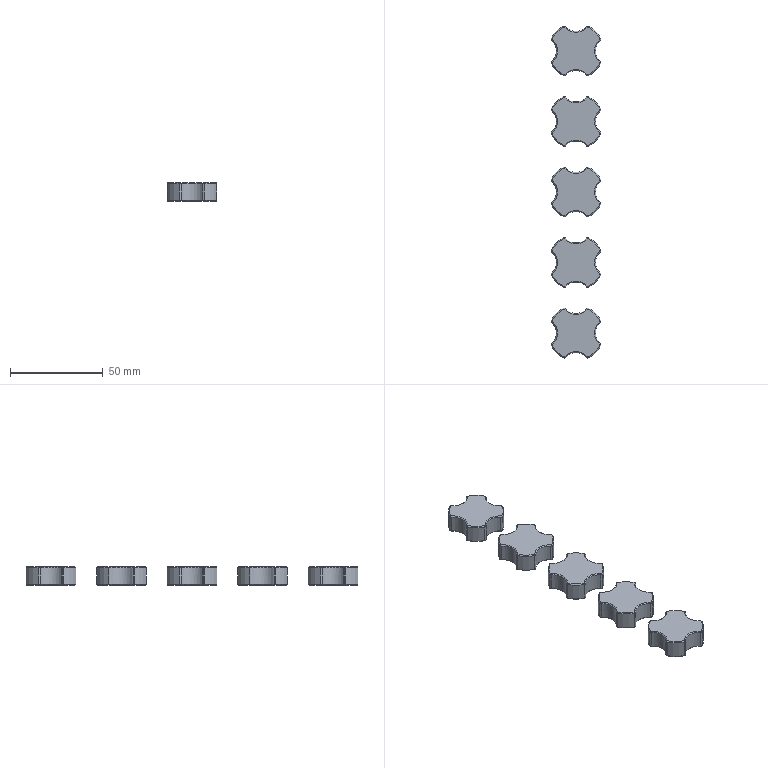NC program | NX | posted with a generic post | part box 26.875 x 178.875 x 10 mm
Lines 1 to 18 of 10509:
N10 G17 G21 G94 G90
(FLOOR_WALL , TOOL : D80)
N12 T19 M6
N14 G54
N16 G17 G0 G90 X-136.438 Y0. S6500 M3
N18 G43 Z30. H19
N20 Z3.
N22 G94 G1 Z0. F1500.
N24 X-131.438
N26 X131.438
N28 X136.438
N30 Z3.
N32 G0 Z30.
N34 M5